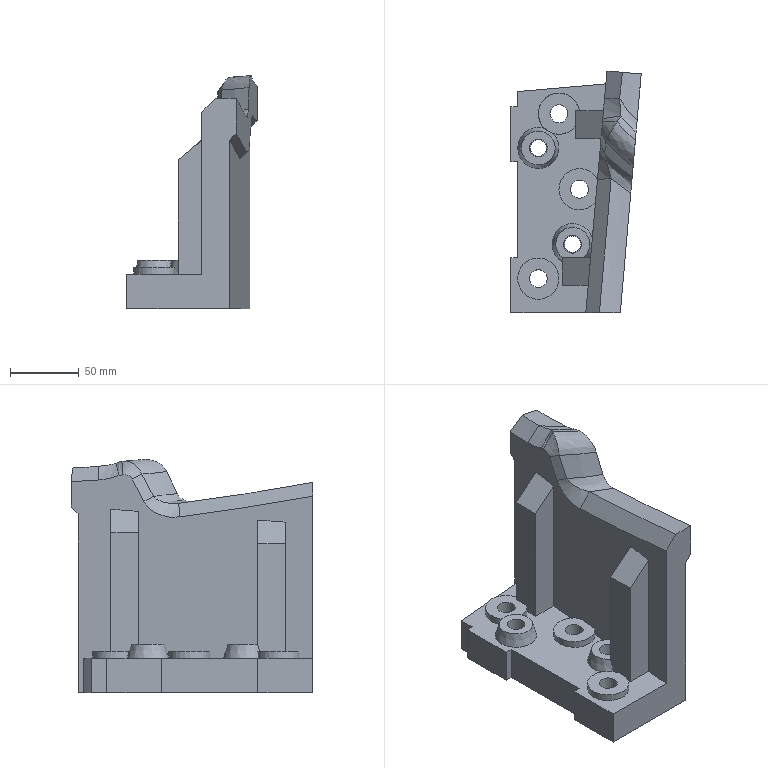Part | NX | features solid 2 | 1 solid | 61 faces | box 94.853 x 175.81 x 169.621 mm | volume 854069 mm3 | plane 34 | spline 15 | cylinder 10 | cone 2 | commonest cylinder face diameters 13 x5 30 x3 12 x2